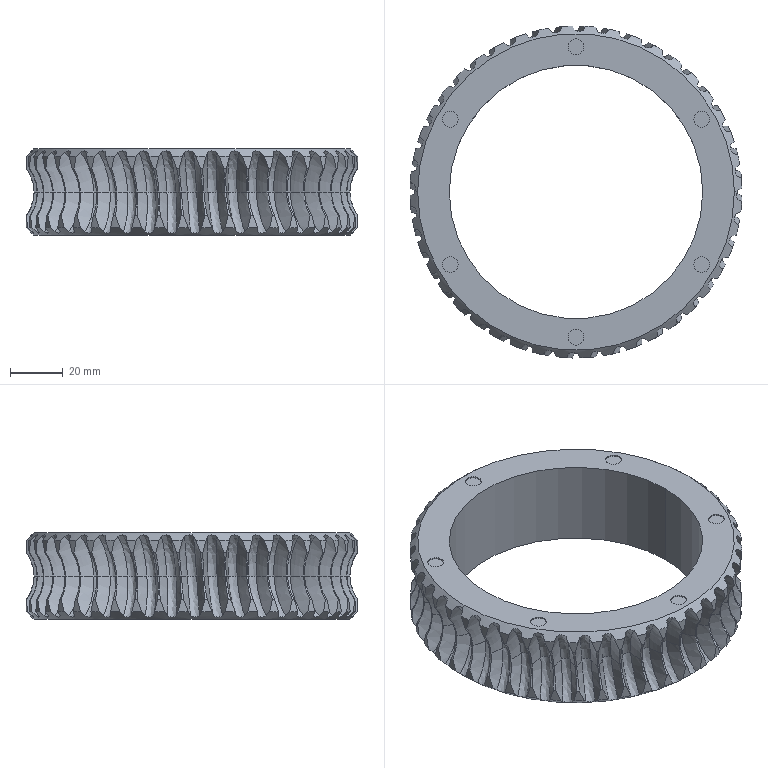Part | SolidWorks | features CirPattern 2, Helix 2, ICE 2, SweepCut 2, Chamfer 1, Extrusion 1, RevCut 1, Scale 1 | 1 solid | 466 faces | box 125.684 x 125.684 x 32.802 mm | volume 115806 mm3 | spline 264 | cylinder 102 | torus 88 | plane 8 | cone 4 | commonest cylinder face diameters 125.715 x88 6 x12 96 x2